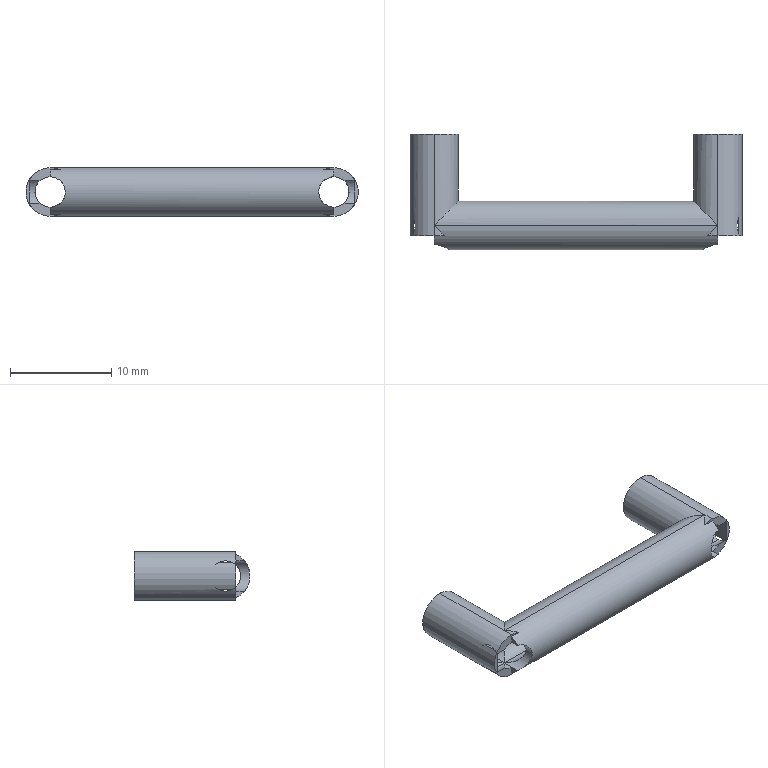Part | SolidWorks | features BaseBody 1 | 1 solid | 38 faces | box 32.8 x 11.4 x 4.8 mm | volume 474.136 mm3 | cylinder 28 | plane 10 | commonest cylinder face diameters 3 x18 4.8 x10
STEP:
#1=CARTESIAN_POINT('',(-14.,-15.,-2.4));
#2=VERTEX_POINT('',#1);
#3=CARTESIAN_POINT('',(-14.,-15.,2.4));
#4=VERTEX_POINT('',#3);
#5=CARTESIAN_POINT('',(-14.,-15.,-2.4));
#6=CARTESIAN_POINT('',(-9.2,-10.2,-2.4));
#7=CARTESIAN_POINT('',(-9.2,-10.2,2.4));
#8=CARTESIAN_POINT('',(-14.,-15.,2.4));
#9=(BOUNDED_CURVE()B_SPLINE_CURVE(3,(#5,#6,#7,#8),.UNSPECIFIED.,.F.,.F.)B_SPLINE_CURVE_WITH_KNOTS((4,4),(4.712,7.854),.UNSPECIFIED.)CURVE()GEOMETRIC_REPRESENTATION_ITEM()RATIONAL_B_SPLINE_CURVE((1.,0.3333,0.3333,1.))REPRESENTATION_ITEM(''));
#10=EDGE_CURVE('',#2,#4,#9,.T.);
#11=ORIENTED_EDGE('',*,*,#10,.T.);
#12=CARTESIAN_POINT('',(14.,-15.,2.4));
#13=VERTEX_POINT('',#12);
#14=CARTESIAN_POINT('',(-14.,-15.,2.4));
#15=DIRECTION('',(1.,0.,0.));
#16=VECTOR('',#15,1000.);
#17=LINE('',#14,#16);
#18=EDGE_CURVE('',#4,#13,#17,.T.);
#19=ORIENTED_EDGE('',*,*,#18,.T.);
#20=CARTESIAN_POINT('',(14.,-15.,-2.4));
#21=VERTEX_POINT('',#20);
#22=CARTESIAN_POINT('',(14.,-15.,2.4));
#23=CARTESIAN_POINT('',(9.2,-10.2,2.4));
#24=CARTESIAN_POINT('',(9.2,-10.2,-2.4));
#25=CARTESIAN_POINT('',(14.,-15.,-2.4));
#26=(BOUNDED_CURVE()B_SPLINE_CURVE(3,(#22,#23,#24,#25),.UNSPECIFIED.,.F.,.F.)B_SPLINE_CURVE_WITH_KNOTS((4,4),(4.712,7.854),.UNSPECIFIED.)CURVE()GEOMETRIC_REPRESENTATION_ITEM()RATIONAL_B_SPLINE_CURVE((1.,0.3333,0.3333,1.))REPRESENTATION_ITEM(''));
#27=EDGE_CURVE('',#13,#21,#26,.T.);
#28=ORIENTED_EDGE('',*,*,#27,.T.);
#29=CARTESIAN_POINT('',(-14.,-15.,-2.4));
#30=DIRECTION('',(1.,0.,0.));
#31=VECTOR('',#30,1000.);
#32=LINE('',#29,#31);
#33=EDGE_CURVE('',#2,#21,#32,.T.);
#34=ORIENTED_EDGE('',*,*,#33,.F.);
#35=EDGE_LOOP('',(#11,#19,#28,#34));
#36=FACE_OUTER_BOUND('',#35,.T.);
#37=CARTESIAN_POINT('',(-14.,-15.,0.));
#38=DIRECTION('',(1.,0.,0.));
#39=DIRECTION('',(0.,0.,-1.));
#40=AXIS2_PLACEMENT_3D('',#37,#38,#39);
#41=CYLINDRICAL_SURFACE('',#40,2.4);
#42=ADVANCED_FACE('',(#36),#41,.T.);
#43=CARTESIAN_POINT('',(-15.,-16.,-1.118));
#44=VERTEX_POINT('',#43);
#45=CARTESIAN_POINT('',(-14.,-16.,-1.5));
#46=VERTEX_POINT('',#45);
#47=CARTESIAN_POINT('',(-14.,-16.,0.));
#48=DIRECTION('',(0.,-1.,0.));
#49=DIRECTION('',(0.,0.,1.));
#50=AXIS2_PLACEMENT_3D('',#47,#48,#49);
#51=CIRCLE('',#50,1.5);
#52=EDGE_CURVE('',#44,#46,#51,.T.);
#53=ORIENTED_EDGE('',*,*,#52,.T.);
#54=CARTESIAN_POINT('',(-14.,-15.,-1.5));
#55=VERTEX_POINT('',#54);
#56=CARTESIAN_POINT('',(-14.,-18.,-1.5));
#57=DIRECTION('',(0.,1.,0.));
#58=VECTOR('',#57,1000.);
#59=LINE('',#56,#58);
#60=EDGE_CURVE('',#46,#55,#59,.T.);
#61=ORIENTED_EDGE('',*,*,#60,.T.);
#62=CARTESIAN_POINT('',(-14.,-15.,-1.5));
#63=CARTESIAN_POINT('',(-14.373,-15.373,-1.5));
#64=CARTESIAN_POINT('',(-14.722,-15.722,-1.367));
#65=CARTESIAN_POINT('',(-15.,-16.,-1.118));
#66=(BOUNDED_CURVE()B_SPLINE_CURVE(3,(#62,#63,#64,#65),.UNSPECIFIED.,.F.,.F.)B_SPLINE_CURVE_WITH_KNOTS((4,4),(1.571,2.301),.UNSPECIFIED.)CURVE()GEOMETRIC_REPRESENTATION_ITEM()RATIONAL_B_SPLINE_CURVE((1.,0.9561,0.9561,1.))REPRESENTATION_ITEM(''));
#67=EDGE_CURVE('',#55,#44,#66,.T.);
#68=ORIENTED_EDGE('',*,*,#67,.T.);
#69=EDGE_LOOP('',(#53,#61,#68));
#70=FACE_OUTER_BOUND('',#69,.T.);
#71=CARTESIAN_POINT('',(-14.,-18.,0.));
#72=DIRECTION('',(0.,1.,0.));
#73=DIRECTION('',(0.,0.,1.));
#74=AXIS2_PLACEMENT_3D('',#71,#72,#73);
#75=CYLINDRICAL_SURFACE('',#74,1.5);
#76=ADVANCED_FACE('',(#70),#75,.F.);
#77=ORIENTED_EDGE('',*,*,#60,.F.);
#78=CARTESIAN_POINT('',(-14.,-16.873,-1.5));
#79=VERTEX_POINT('',#78);
#80=CARTESIAN_POINT('',(-14.,-15.,-1.5));
#81=DIRECTION('',(0.,-1.,0.));
#82=VECTOR('',#81,1000.);
#83=LINE('',#80,#82);
#84=EDGE_CURVE('',#46,#79,#83,.T.);
#85=ORIENTED_EDGE('',*,*,#84,.T.);
#86=CARTESIAN_POINT('',(-14.,-16.873,1.5));
#87=VERTEX_POINT('',#86);
#88=CARTESIAN_POINT('',(-14.,-16.873,1.5));
#89=CARTESIAN_POINT('',(-13.898,-16.873,1.5));
#90=CARTESIAN_POINT('',(-13.798,-16.882,1.49));
#91=CARTESIAN_POINT('',(-13.603,-16.913,1.45));
#92=CARTESIAN_POINT('',(-13.507,-16.935,1.42));
#93=CARTESIAN_POINT('',(-13.238,-17.015,1.307));
#94=CARTESIAN_POINT('',(-13.077,-17.085,1.197));
#95=CARTESIAN_POINT('',(-12.874,-17.185,0.9958));
#96=CARTESIAN_POINT('',(-12.812,-17.218,0.921));
#97=CARTESIAN_POINT('',(-12.704,-17.278,0.7615));
#98=CARTESIAN_POINT('',(-12.658,-17.304,0.6768));
#99=CARTESIAN_POINT('',(-12.581,-17.35,0.4963));
#100=CARTESIAN_POINT('',(-12.551,-17.369,0.3994));
#101=CARTESIAN_POINT('',(-12.511,-17.393,0.2039));
#102=CARTESIAN_POINT('',(-12.5,-17.4,0.1043));
#103=CARTESIAN_POINT('',(-12.5,-17.4,-0.2004));
#104=CARTESIAN_POINT('',(-12.542,-17.373,-0.4024));
#105=CARTESIAN_POINT('',(-12.695,-17.282,-0.7658));
#106=CARTESIAN_POINT('',(-12.806,-17.218,-0.9283));
#107=CARTESIAN_POINT('',(-13.077,-17.085,-1.197));
#108=CARTESIAN_POINT('',(-13.237,-17.016,-1.306));
#109=CARTESIAN_POINT('',(-13.506,-16.936,-1.42));
#110=CARTESIAN_POINT('',(-13.602,-16.913,-1.45));
#111=CARTESIAN_POINT('',(-13.798,-16.882,-1.49));
#112=CARTESIAN_POINT('',(-13.898,-16.873,-1.5));
#113=CARTESIAN_POINT('',(-14.,-16.873,-1.5));
#114=B_SPLINE_CURVE_WITH_KNOTS('',3,(#88,#89,#90,#91,#92,#93,#94,#95,#96,#97,#98,#99,#100,#101,#102,#103,#104,#105,#106,#107,#108,#109,#110,#111,#112,#113),.UNSPECIFIED.,.F.,.F.,(4,2,2,2,2,2,2,2,2,2,2,2,4),(0.,0.0003015,0.0006029,0.001206,0.001507,0.001809,0.00211,0.002412,0.003015,0.003617,0.00422,0.004522,0.004823),.UNSPECIFIED.);
#115=EDGE_CURVE('',#87,#79,#114,.T.);
#116=ORIENTED_EDGE('',*,*,#115,.F.);
#117=CARTESIAN_POINT('',(-14.,-16.,1.5));
#118=VERTEX_POINT('',#117);
#119=CARTESIAN_POINT('',(-14.,-18.,1.5));
#120=DIRECTION('',(0.,-1.,0.));
#121=VECTOR('',#120,1000.);
#122=LINE('',#119,#121);
#123=EDGE_CURVE('',#118,#87,#122,.T.);
#124=ORIENTED_EDGE('',*,*,#123,.F.);
#125=CARTESIAN_POINT('',(-14.,-15.,1.5));
#126=VERTEX_POINT('',#125);
#127=CARTESIAN_POINT('',(-14.,-18.,1.5));
#128=DIRECTION('',(0.,1.,0.));
#129=VECTOR('',#128,1000.);
#130=LINE('',#127,#129);
#131=EDGE_CURVE('',#118,#126,#130,.T.);
#132=ORIENTED_EDGE('',*,*,#131,.T.);
#133=CARTESIAN_POINT('',(-14.,-15.,-1.5));
#134=CARTESIAN_POINT('',(-11.,-18.,-1.5));
#135=CARTESIAN_POINT('',(-11.,-18.,1.5));
#136=CARTESIAN_POINT('',(-14.,-15.,1.5));
#137=(BOUNDED_CURVE()B_SPLINE_CURVE(3,(#133,#134,#135,#136),.UNSPECIFIED.,.F.,.F.)B_SPLINE_CURVE_WITH_KNOTS((4,4),(4.712,7.854),.UNSPECIFIED.)CURVE()GEOMETRIC_REPRESENTATION_ITEM()RATIONAL_B_SPLINE_CURVE((1.,0.3333,0.3333,1.))REPRESENTATION_ITEM(''));
#138=EDGE_CURVE('',#55,#126,#137,.T.);
#139=ORIENTED_EDGE('',*,*,#138,.F.);
#140=EDGE_LOOP('',(#77,#85,#116,#124,#132,#139));
#141=FACE_OUTER_BOUND('',#140,.T.);
#142=CARTESIAN_POINT('',(-14.,-18.,0.));
#143=DIRECTION('',(0.,1.,0.));
#144=DIRECTION('',(0.,0.,1.));
#145=AXIS2_PLACEMENT_3D('',#142,#143,#144);
#146=CYLINDRICAL_SURFACE('',#145,1.5);
#147=ADVANCED_FACE('',(#141),#146,.F.);
#148=CARTESIAN_POINT('',(-13.,-16.,-2.182));
#149=VERTEX_POINT('',#148);
#150=CARTESIAN_POINT('',(-14.,-16.,-2.4));
#151=VERTEX_POINT('',#150);
#152=CARTESIAN_POINT('',(-14.,-16.,0.));
#153=DIRECTION('',(0.,1.,0.));
#154=DIRECTION('',(0.,0.,1.));
#155=AXIS2_PLACEMENT_3D('',#152,#153,#154);
#156=CIRCLE('',#155,2.4);
#157=EDGE_CURVE('',#149,#151,#156,.T.);
#158=ORIENTED_EDGE('',*,*,#157,.T.);
#159=CARTESIAN_POINT('',(-14.,-16.,-2.4));
#160=DIRECTION('',(0.,1.,0.));
#161=VECTOR('',#160,1000.);
#162=LINE('',#159,#161);
#163=EDGE_CURVE('',#151,#2,#162,.T.);
#164=ORIENTED_EDGE('',*,*,#163,.T.);
#165=CARTESIAN_POINT('',(-14.,-15.,-2.4));
#166=CARTESIAN_POINT('',(-13.654,-15.346,-2.4));
#167=CARTESIAN_POINT('',(-13.315,-15.685,-2.326));
#168=CARTESIAN_POINT('',(-13.,-16.,-2.182));
#169=(BOUNDED_CURVE()B_SPLINE_CURVE(3,(#165,#166,#167,#168),.UNSPECIFIED.,.F.,.F.)B_SPLINE_CURVE_WITH_KNOTS((4,4),(4.712,5.142),.UNSPECIFIED.)CURVE()GEOMETRIC_REPRESENTATION_ITEM()RATIONAL_B_SPLINE_CURVE((1.,0.9847,0.9847,1.))REPRESENTATION_ITEM(''));
#170=EDGE_CURVE('',#2,#149,#169,.T.);
#171=ORIENTED_EDGE('',*,*,#170,.T.);
#172=EDGE_LOOP('',(#158,#164,#171));
#173=FACE_OUTER_BOUND('',#172,.T.);
#174=CARTESIAN_POINT('',(-14.,-16.,0.));
#175=DIRECTION('',(0.,1.,0.));
#176=DIRECTION('',(0.,0.,1.));
#177=AXIS2_PLACEMENT_3D('',#174,#175,#176);
#178=CYLINDRICAL_SURFACE('',#177,2.4);
#179=ADVANCED_FACE('',(#173),#178,.T.);
#180=ORIENTED_EDGE('',*,*,#10,.F.);
#181=CARTESIAN_POINT('',(-14.,-6.,-2.4));
#182=VERTEX_POINT('',#181);
#183=CARTESIAN_POINT('',(-14.,-16.,-2.4));
#184=DIRECTION('',(0.,1.,0.));
#185=VECTOR('',#184,1000.);
#186=LINE('',#183,#185);
#187=EDGE_CURVE('',#2,#182,#186,.T.);
#188=ORIENTED_EDGE('',*,*,#187,.T.);
#189=CARTESIAN_POINT('',(-14.,-6.,2.4));
#190=VERTEX_POINT('',#189);
#191=CARTESIAN_POINT('',(-14.,-6.,0.));
#192=DIRECTION('',(0.,-1.,0.));
#193=DIRECTION('',(0.,0.,1.));
#194=AXIS2_PLACEMENT_3D('',#191,#192,#193);
#195=CIRCLE('',#194,2.4);
#196=EDGE_CURVE('',#182,#190,#195,.T.);
#197=ORIENTED_EDGE('',*,*,#196,.T.);
#198=CARTESIAN_POINT('',(-14.,-16.,2.4));
#199=DIRECTION('',(0.,1.,0.));
#200=VECTOR('',#199,1000.);
#201=LINE('',#198,#200);
#202=EDGE_CURVE('',#4,#190,#201,.T.);
#203=ORIENTED_EDGE('',*,*,#202,.F.);
#204=EDGE_LOOP('',(#180,#188,#197,#203));
#205=FACE_OUTER_BOUND('',#204,.T.);
#206=CARTESIAN_POINT('',(-14.,-16.,0.));
#207=DIRECTION('',(0.,1.,0.));
#208=DIRECTION('',(0.,0.,1.));
#209=AXIS2_PLACEMENT_3D('',#206,#207,#208);
#210=CYLINDRICAL_SURFACE('',#209,2.4);
#211=ADVANCED_FACE('',(#205),#210,.T.);
#212=ORIENTED_EDGE('',*,*,#163,.F.);
#213=CARTESIAN_POINT('',(-14.,-16.,2.4));
#214=VERTEX_POINT('',#213);
#215=CARTESIAN_POINT('',(-14.,-16.,0.));
#216=DIRECTION('',(0.,1.,0.));
#217=DIRECTION('',(0.,0.,1.));
#218=AXIS2_PLACEMENT_3D('',#215,#216,#217);
#219=CIRCLE('',#218,2.4);
#220=EDGE_CURVE('',#151,#214,#219,.T.);
#221=ORIENTED_EDGE('',*,*,#220,.T.);
#222=CARTESIAN_POINT('',(-14.,-16.,2.4));
#223=DIRECTION('',(0.,1.,0.));
#224=VECTOR('',#223,1000.);
#225=LINE('',#222,#224);
#226=EDGE_CURVE('',#214,#4,#225,.T.);
#227=ORIENTED_EDGE('',*,*,#226,.T.);
#228=ORIENTED_EDGE('',*,*,#202,.T.);
#229=CARTESIAN_POINT('',(-14.,-6.,0.));
#230=DIRECTION('',(0.,-1.,0.));
#231=DIRECTION('',(0.,0.,1.));
#232=AXIS2_PLACEMENT_3D('',#229,#230,#231);
#233=CIRCLE('',#232,2.4);
#234=EDGE_CURVE('',#190,#182,#233,.T.);
#235=ORIENTED_EDGE('',*,*,#234,.T.);
#236=ORIENTED_EDGE('',*,*,#187,.F.);
#237=EDGE_LOOP('',(#212,#221,#227,#228,#235,#236));
#238=FACE_OUTER_BOUND('',#237,.T.);
#239=CARTESIAN_POINT('',(-16.,-14.3,1.327));
#240=VERTEX_POINT('',#239);
#241=CARTESIAN_POINT('',(-16.,-15.7,1.327));
#242=VERTEX_POINT('',#241);
#243=CARTESIAN_POINT('',(-16.,-15.,1.327));
#244=DIRECTION('',(0.,-1.,0.));
#245=VECTOR('',#244,1000.);
#246=LINE('',#243,#245);
#247=EDGE_CURVE('',#240,#242,#246,.T.);
#248=ORIENTED_EDGE('',*,*,#247,.F.);
#249=CARTESIAN_POINT('',(-15.873,-15.,1.5));
#250=VERTEX_POINT('',#249);
#251=CARTESIAN_POINT('',(-16.,-14.3,1.327));
#252=CARTESIAN_POINT('',(-15.963,-14.405,1.382));
#253=CARTESIAN_POINT('',(-15.931,-14.517,1.425));
#254=CARTESIAN_POINT('',(-15.886,-14.753,1.485));
#255=CARTESIAN_POINT('',(-15.873,-14.877,1.5));
#256=CARTESIAN_POINT('',(-15.873,-15.,1.5));
#257=B_SPLINE_CURVE_WITH_KNOTS('',3,(#251,#252,#253,#254,#255,#256),.UNSPECIFIED.,.F.,.F.,(4,2,4),(0.,0.00037,0.0007401),.UNSPECIFIED.);
#258=EDGE_CURVE('',#240,#250,#257,.T.);
#259=ORIENTED_EDGE('',*,*,#258,.T.);
#260=CARTESIAN_POINT('',(-15.873,-15.,1.5));
#261=CARTESIAN_POINT('',(-15.873,-15.123,1.5));
#262=CARTESIAN_POINT('',(-15.886,-15.247,1.484));
#263=CARTESIAN_POINT('',(-15.931,-15.482,1.426));
#264=CARTESIAN_POINT('',(-15.963,-15.595,1.382));
#265=CARTESIAN_POINT('',(-16.,-15.7,1.327));
#266=B_SPLINE_CURVE_WITH_KNOTS('',3,(#260,#261,#262,#263,#264,#265),.UNSPECIFIED.,.F.,.F.,(4,2,4),(0.0007401,0.001109,0.001477),.UNSPECIFIED.);
#267=EDGE_CURVE('',#250,#242,#266,.T.);
#268=ORIENTED_EDGE('',*,*,#267,.T.);
#269=EDGE_LOOP('',(#248,#259,#268));
#270=FACE_BOUND('',#269,.T.);
#271=CARTESIAN_POINT('',(-16.,-15.7,-1.327));
#272=VERTEX_POINT('',#271);
#273=CARTESIAN_POINT('',(-15.873,-15.,-1.5));
#274=VERTEX_POINT('',#273);
#275=CARTESIAN_POINT('',(-16.,-15.7,-1.327));
#276=CARTESIAN_POINT('',(-15.963,-15.595,-1.382));
#277=CARTESIAN_POINT('',(-15.931,-15.483,-1.425));
#278=CARTESIAN_POINT('',(-15.886,-15.247,-1.485));
#279=CARTESIAN_POINT('',(-15.873,-15.123,-1.5));
#280=CARTESIAN_POINT('',(-15.873,-15.,-1.5));
#281=B_SPLINE_CURVE_WITH_KNOTS('',3,(#275,#276,#277,#278,#279,#280),.UNSPECIFIED.,.F.,.F.,(4,2,4),(0.,0.00037,0.0007401),.UNSPECIFIED.);
#282=EDGE_CURVE('',#272,#274,#281,.T.);
#283=ORIENTED_EDGE('',*,*,#282,.T.);
#284=CARTESIAN_POINT('',(-16.,-14.3,-1.327));
#285=VERTEX_POINT('',#284);
#286=CARTESIAN_POINT('',(-15.873,-15.,-1.5));
#287=CARTESIAN_POINT('',(-15.873,-14.877,-1.5));
#288=CARTESIAN_POINT('',(-15.886,-14.753,-1.484));
#289=CARTESIAN_POINT('',(-15.931,-14.518,-1.426));
#290=CARTESIAN_POINT('',(-15.963,-14.405,-1.382));
#291=CARTESIAN_POINT('',(-16.,-14.3,-1.327));
#292=B_SPLINE_CURVE_WITH_KNOTS('',3,(#286,#287,#288,#289,#290,#291),.UNSPECIFIED.,.F.,.F.,(4,2,4),(0.0007401,0.001109,0.001477),.UNSPECIFIED.);
#293=EDGE_CURVE('',#274,#285,#292,.T.);
#294=ORIENTED_EDGE('',*,*,#293,.T.);
#295=CARTESIAN_POINT('',(-16.,-16.,-1.327));
#296=DIRECTION('',(0.,-1.,0.));
#297=VECTOR('',#296,1000.);
#298=LINE('',#295,#297);
#299=EDGE_CURVE('',#285,#272,#298,.T.);
#300=ORIENTED_EDGE('',*,*,#299,.T.);
#301=EDGE_LOOP('',(#283,#294,#300));
#302=FACE_BOUND('',#301,.T.);
#303=CARTESIAN_POINT('',(-14.,-16.,0.));
#304=DIRECTION('',(0.,1.,0.));
#305=DIRECTION('',(0.,0.,1.));
#306=AXIS2_PLACEMENT_3D('',#303,#304,#305);
#307=CYLINDRICAL_SURFACE('',#306,2.4);
#308=ADVANCED_FACE('',(#238,#270,#302),#307,.T.);
#309=CARTESIAN_POINT('',(16.,-15.7,1.327));
#310=VERTEX_POINT('',#309);
#311=CARTESIAN_POINT('',(15.873,-15.,1.5));
#312=VERTEX_POINT('',#311);
#313=CARTESIAN_POINT('',(16.,-15.7,1.327));
#314=CARTESIAN_POINT('',(15.963,-15.595,1.382));
#315=CARTESIAN_POINT('',(15.931,-15.483,1.425));
#316=CARTESIAN_POINT('',(15.886,-15.247,1.485));
#317=CARTESIAN_POINT('',(15.873,-15.123,1.5));
#318=CARTESIAN_POINT('',(15.873,-15.,1.5));
#319=B_SPLINE_CURVE_WITH_KNOTS('',3,(#313,#314,#315,#316,#317,#318),.UNSPECIFIED.,.F.,.F.,(4,2,4),(0.,0.00037,0.0007401),.UNSPECIFIED.);
#320=EDGE_CURVE('',#310,#312,#319,.T.);
#321=ORIENTED_EDGE('',*,*,#320,.T.);
#322=CARTESIAN_POINT('',(16.,-14.3,1.327));
#323=VERTEX_POINT('',#322);
#324=CARTESIAN_POINT('',(15.873,-15.,1.5));
#325=CARTESIAN_POINT('',(15.873,-14.877,1.5));
#326=CARTESIAN_POINT('',(15.886,-14.753,1.484));
#327=CARTESIAN_POINT('',(15.931,-14.518,1.426));
#328=CARTESIAN_POINT('',(15.963,-14.405,1.382));
#329=CARTESIAN_POINT('',(16.,-14.3,1.327));
#330=B_SPLINE_CURVE_WITH_KNOTS('',3,(#324,#325,#326,#327,#328,#329),.UNSPECIFIED.,.F.,.F.,(4,2,4),(0.0007401,0.001109,0.001477),.UNSPECIFIED.);
#331=EDGE_CURVE('',#312,#323,#330,.T.);
#332=ORIENTED_EDGE('',*,*,#331,.T.);
#333=CARTESIAN_POINT('',(16.,-16.,1.327));
#334=DIRECTION('',(0.,-1.,0.));
#335=VECTOR('',#334,1000.);
#336=LINE('',#333,#335);
#337=EDGE_CURVE('',#323,#310,#336,.T.);
#338=ORIENTED_EDGE('',*,*,#337,.T.);
#339=EDGE_LOOP('',(#321,#332,#338));
#340=FACE_BOUND('',#339,.T.);
#341=CARTESIAN_POINT('',(16.,-14.3,-1.327));
#342=VERTEX_POINT('',#341);
#343=CARTESIAN_POINT('',(15.873,-15.,-1.5));
#344=VERTEX_POINT('',#343);
#345=CARTESIAN_POINT('',(16.,-14.3,-1.327));
#346=CARTESIAN_POINT('',(15.963,-14.405,-1.382));
#347=CARTESIAN_POINT('',(15.931,-14.517,-1.425));
#348=CARTESIAN_POINT('',(15.886,-14.753,-1.485));
#349=CARTESIAN_POINT('',(15.873,-14.877,-1.5));
#350=CARTESIAN_POINT('',(15.873,-15.,-1.5));
#351=B_SPLINE_CURVE_WITH_KNOTS('',3,(#345,#346,#347,#348,#349,#350),.UNSPECIFIED.,.F.,.F.,(4,2,4),(0.,0.00037,0.0007401),.UNSPECIFIED.);
#352=EDGE_CURVE('',#342,#344,#351,.T.);
#353=ORIENTED_EDGE('',*,*,#352,.T.);
#354=CARTESIAN_POINT('',(16.,-15.7,-1.327));
#355=VERTEX_POINT('',#354);
#356=CARTESIAN_POINT('',(15.873,-15.,-1.5));
#357=CARTESIAN_POINT('',(15.873,-15.123,-1.5));
#358=CARTESIAN_POINT('',(15.886,-15.247,-1.484));
#359=CARTESIAN_POINT('',(15.931,-15.482,-1.426));
#360=CARTESIAN_POINT('',(15.963,-15.595,-1.382));
#361=CARTESIAN_POINT('',(16.,-15.7,-1.327));
#362=B_SPLINE_CURVE_WITH_KNOTS('',3,(#356,#357,#358,#359,#360,#361),.UNSPECIFIED.,.F.,.F.,(4,2,4),(0.0007401,0.001109,0.001477),.UNSPECIFIED.);
#363=EDGE_CURVE('',#344,#355,#362,.T.);
#364=ORIENTED_EDGE('',*,*,#363,.T.);
#365=CARTESIAN_POINT('',(16.,-16.,-1.327));
#366=DIRECTION('',(0.,1.,0.));
#367=VECTOR('',#366,1000.);
#368=LINE('',#365,#367);
#369=EDGE_CURVE('',#355,#342,#368,.T.);
#370=ORIENTED_EDGE('',*,*,#369,.T.);
#371=EDGE_LOOP('',(#353,#364,#370));
#372=FACE_BOUND('',#371,.T.);
#373=CARTESIAN_POINT('',(14.,-16.,2.4));
#374=VERTEX_POINT('',#373);
#375=CARTESIAN_POINT('',(14.,-16.,-2.4));
#376=VERTEX_POINT('',#375);
#377=CARTESIAN_POINT('',(14.,-16.,0.));
#378=DIRECTION('',(0.,1.,0.));
#379=DIRECTION('',(0.,0.,1.));
#380=AXIS2_PLACEMENT_3D('',#377,#378,#379);
#381=CIRCLE('',#380,2.4);
#382=EDGE_CURVE('',#374,#376,#381,.T.);
#383=ORIENTED_EDGE('',*,*,#382,.T.);
#384=CARTESIAN_POINT('',(14.,-16.,-2.4));
#385=DIRECTION('',(0.,1.,0.));
#386=VECTOR('',#385,1000.);
#387=LINE('',#384,#386);
#388=EDGE_CURVE('',#376,#21,#387,.T.);
#389=ORIENTED_EDGE('',*,*,#388,.T.);
#390=CARTESIAN_POINT('',(14.,-6.,-2.4));
#391=VERTEX_POINT('',#390);
#392=CARTESIAN_POINT('',(14.,-16.,-2.4));
#393=DIRECTION('',(0.,1.,0.));
#394=VECTOR('',#393,1000.);
#395=LINE('',#392,#394);
#396=EDGE_CURVE('',#21,#391,#395,.T.);
#397=ORIENTED_EDGE('',*,*,#396,.T.);
#398=CARTESIAN_POINT('',(14.,-6.,2.4));
#399=VERTEX_POINT('',#398);
#400=CARTESIAN_POINT('',(14.,-6.,0.));
#401=DIRECTION('',(0.,-1.,0.));
#402=DIRECTION('',(0.,0.,1.));
#403=AXIS2_PLACEMENT_3D('',#400,#401,#402);
#404=CIRCLE('',#403,2.4);
#405=EDGE_CURVE('',#391,#399,#404,.T.);
#406=ORIENTED_EDGE('',*,*,#405,.T.);
#407=CARTESIAN_POINT('',(14.,-16.,2.4));
#408=DIRECTION('',(0.,1.,0.));
#409=VECTOR('',#408,1000.);
#410=LINE('',#407,#409);
#411=EDGE_CURVE('',#13,#399,#410,.T.);
#412=ORIENTED_EDGE('',*,*,#411,.F.);
#413=CARTESIAN_POINT('',(14.,-16.,2.4));
#414=DIRECTION('',(0.,1.,0.));
#415=VECTOR('',#414,1000.);
#416=LINE('',#413,#415);
#417=EDGE_CURVE('',#374,#13,#416,.T.);
#418=ORIENTED_EDGE('',*,*,#417,.F.);
#419=EDGE_LOOP('',(#383,#389,#397,#406,#412,#418));
#420=FACE_OUTER_BOUND('',#419,.T.);
#421=CARTESIAN_POINT('',(14.,-16.,0.));
#422=DIRECTION('',(0.,1.,0.));
#423=DIRECTION('',(0.,0.,1.));
#424=AXIS2_PLACEMENT_3D('',#421,#422,#423);
#425=CYLINDRICAL_SURFACE('',#424,2.4);
#426=ADVANCED_FACE('',(#340,#372,#420),#425,.T.);
#427=ORIENTED_EDGE('',*,*,#388,.F.);
#428=CARTESIAN_POINT('',(13.,-16.,-2.182));
#429=VERTEX_POINT('',#428);
#430=CARTESIAN_POINT('',(14.,-16.,0.));
#431=DIRECTION('',(0.,1.,0.));
#432=DIRECTION('',(0.,0.,1.));
#433=AXIS2_PLACEMENT_3D('',#430,#431,#432);
#434=CIRCLE('',#433,2.4);
#435=EDGE_CURVE('',#376,#429,#434,.T.);
#436=ORIENTED_EDGE('',*,*,#435,.T.);
#437=CARTESIAN_POINT('',(14.,-15.,-2.4));
#438=CARTESIAN_POINT('',(13.654,-15.346,-2.4));
#439=CARTESIAN_POINT('',(13.315,-15.685,-2.326));
#440=CARTESIAN_POINT('',(13.,-16.,-2.182));
#441=(BOUNDED_CURVE()B_SPLINE_CURVE(3,(#437,#438,#439,#440),.UNSPECIFIED.,.F.,.F.)B_SPLINE_CURVE_WITH_KNOTS((4,4),(1.571,2.001),.UNSPECIFIED.)CURVE()GEOMETRIC_REPRESENTATION_ITEM()RATIONAL_B_SPLINE_CURVE((1.,0.9847,0.9847,1.))REPRESENTATION_ITEM(''));
#442=EDGE_CURVE('',#21,#429,#441,.T.);
#443=ORIENTED_EDGE('',*,*,#442,.F.);
#444=EDGE_LOOP('',(#427,#436,#443));
#445=FACE_OUTER_BOUND('',#444,.T.);
#446=CARTESIAN_POINT('',(14.,-16.,0.));
#447=DIRECTION('',(0.,1.,0.));
#448=DIRECTION('',(0.,0.,1.));
#449=AXIS2_PLACEMENT_3D('',#446,#447,#448);
#450=CYLINDRICAL_SURFACE('',#449,2.4);
#451=ADVANCED_FACE('',(#445),#450,.T.);
#452=CARTESIAN_POINT('',(13.,-16.,2.182));
#453=VERTEX_POINT('',#452);
#454=CARTESIAN_POINT('',(14.,-16.,0.));
#455=DIRECTION('',(0.,1.,0.));
#456=DIRECTION('',(0.,0.,1.));
#457=AXIS2_PLACEMENT_3D('',#454,#455,#456);
#458=CIRCLE('',#457,2.4);
#459=EDGE_CURVE('',#453,#374,#458,.T.);
#460=ORIENTED_EDGE('',*,*,#459,.T.);
#461=ORIENTED_EDGE('',*,*,#417,.T.);
#462=CARTESIAN_POINT('',(13.,-16.,2.182));
#463=CARTESIAN_POINT('',(13.315,-15.685,2.326));
#464=CARTESIAN_POINT('',(13.654,-15.346,2.4));
#465=CARTESIAN_POINT('',(14.,-15.,2.4));
#466=(BOUNDED_CURVE()B_SPLINE_CURVE(3,(#462,#463,#464,#465),.UNSPECIFIED.,.F.,.F.)B_SPLINE_CURVE_WITH_KNOTS((4,4),(4.283,4.712),.UNSPECIFIED.)CURVE()GEOMETRIC_REPRESENTATION_ITEM()RATIONAL_B_SPLINE_CURVE((1.,0.9847,0.9847,1.))REPRESENTATION_ITEM(''));
#467=EDGE_CURVE('',#453,#13,#466,.T.);
#468=ORIENTED_EDGE('',*,*,#467,.F.);
#469=EDGE_LOOP('',(#460,#461,#468));
#470=FACE_OUTER_BOUND('',#469,.T.);
#471=CARTESIAN_POINT('',(14.,-16.,0.));
#472=DIRECTION('',(0.,1.,0.));
#473=DIRECTION('',(0.,0.,1.));
#474=AXIS2_PLACEMENT_3D('',#471,#472,#473);
#475=CYLINDRICAL_SURFACE('',#474,2.4);
#476=ADVANCED_FACE('',(#470),#475,.T.);
#477=CARTESIAN_POINT('',(14.,-16.,-1.5));
#478=VERTEX_POINT('',#477);
#479=CARTESIAN_POINT('',(14.,-16.873,-1.5));
#480=VERTEX_POINT('',#479);
#481=CARTESIAN_POINT('',(14.,-18.,-1.5));
#482=DIRECTION('',(0.,-1.,0.));
#483=VECTOR('',#482,1000.);
#484=LINE('',#481,#483);
#485=EDGE_CURVE('',#478,#480,#484,.T.);
#486=ORIENTED_EDGE('',*,*,#485,.F.);
#487=CARTESIAN_POINT('',(14.,-15.,-1.5));
#488=VERTEX_POINT('',#487);
#489=CARTESIAN_POINT('',(14.,-18.,-1.5));
#490=DIRECTION('',(0.,1.,0.));
#491=VECTOR('',#490,1000.);
#492=LINE('',#489,#491);
#493=EDGE_CURVE('',#478,#488,#492,.T.);
#494=ORIENTED_EDGE('',*,*,#493,.T.);
#495=CARTESIAN_POINT('',(14.,-15.,1.5));
#496=VERTEX_POINT('',#495);
#497=CARTESIAN_POINT('',(14.,-15.,1.5));
#498=CARTESIAN_POINT('',(11.,-18.,1.5));
#499=CARTESIAN_POINT('',(11.,-18.,-1.5));
#500=CARTESIAN_POINT('',(14.,-15.,-1.5));
#501=(BOUNDED_CURVE()B_SPLINE_CURVE(3,(#497,#498,#499,#500),.UNSPECIFIED.,.F.,.F.)B_SPLINE_CURVE_WITH_KNOTS((4,4),(1.571,4.712),.UNSPECIFIED.)CURVE()GEOMETRIC_REPRESENTATION_ITEM()RATIONAL_B_SPLINE_CURVE((1.,0.3333,0.3333,1.))REPRESENTATION_ITEM(''));
#502=EDGE_CURVE('',#496,#488,#501,.T.);
#503=ORIENTED_EDGE('',*,*,#502,.F.);
#504=CARTESIAN_POINT('',(14.,-16.,1.5));
#505=VERTEX_POINT('',#504);
#506=CARTESIAN_POINT('',(14.,-18.,1.5));
#507=DIRECTION('',(0.,1.,0.));
#508=VECTOR('',#507,1000.);
#509=LINE('',#506,#508);
#510=EDGE_CURVE('',#505,#496,#509,.T.);
#511=ORIENTED_EDGE('',*,*,#510,.F.);
#512=CARTESIAN_POINT('',(14.,-16.873,1.5));
#513=VERTEX_POINT('',#512);
#514=CARTESIAN_POINT('',(14.,-15.,1.5));
#515=DIRECTION('',(0.,1.,0.));
#516=VECTOR('',#515,1000.);
#517=LINE('',#514,#516);
#518=EDGE_CURVE('',#513,#505,#517,.T.);
#519=ORIENTED_EDGE('',*,*,#518,.F.);
#520=CARTESIAN_POINT('',(14.,-16.873,-1.5));
#521=CARTESIAN_POINT('',(13.898,-16.873,-1.5));
#522=CARTESIAN_POINT('',(13.798,-16.882,-1.49));
#523=CARTESIAN_POINT('',(13.603,-16.913,-1.45));
#524=CARTESIAN_POINT('',(13.507,-16.935,-1.42));
#525=CARTESIAN_POINT('',(13.238,-17.015,-1.307));
#526=CARTESIAN_POINT('',(13.077,-17.085,-1.197));
#527=CARTESIAN_POINT('',(12.874,-17.185,-0.9958));
#528=CARTESIAN_POINT('',(12.812,-17.218,-0.921));
#529=CARTESIAN_POINT('',(12.704,-17.278,-0.7615));
#530=CARTESIAN_POINT('',(12.658,-17.304,-0.6768));
#531=CARTESIAN_POINT('',(12.581,-17.35,-0.4963));
#532=CARTESIAN_POINT('',(12.551,-17.369,-0.3994));
#533=CARTESIAN_POINT('',(12.511,-17.393,-0.2039));
#534=CARTESIAN_POINT('',(12.5,-17.4,-0.1043));
#535=CARTESIAN_POINT('',(12.5,-17.4,0.2004));
#536=CARTESIAN_POINT('',(12.542,-17.373,0.4024));
#537=CARTESIAN_POINT('',(12.695,-17.282,0.7658));
#538=CARTESIAN_POINT('',(12.806,-17.218,0.9283));
#539=CARTESIAN_POINT('',(13.077,-17.085,1.197));
#540=CARTESIAN_POINT('',(13.237,-17.016,1.306));
#541=CARTESIAN_POINT('',(13.506,-16.936,1.42));
#542=CARTESIAN_POINT('',(13.602,-16.913,1.45));
#543=CARTESIAN_POINT('',(13.798,-16.882,1.49));
#544=CARTESIAN_POINT('',(13.898,-16.873,1.5));
#545=CARTESIAN_POINT('',(14.,-16.873,1.5));
#546=B_SPLINE_CURVE_WITH_KNOTS('',3,(#520,#521,#522,#523,#524,#525,#526,#527,#528,#529,#530,#531,#532,#533,#534,#535,#536,#537,#538,#539,#540,#541,#542,#543,#544,#545),.UNSPECIFIED.,.F.,.F.,(4,2,2,2,2,2,2,2,2,2,2,2,4),(0.,0.0003015,0.0006029,0.001206,0.001507,0.001809,0.00211,0.002412,0.003015,0.003617,0.00422,0.004522,0.004823),.UNSPECIFIED.);
#547=EDGE_CURVE('',#480,#513,#546,.T.);
#548=ORIENTED_EDGE('',*,*,#547,.F.);
#549=EDGE_LOOP('',(#486,#494,#503,#511,#519,#548));
#550=FACE_OUTER_BOUND('',#549,.T.);
#551=CARTESIAN_POINT('',(14.,-18.,0.));
#552=DIRECTION('',(0.,1.,0.));
#553=DIRECTION('',(0.,0.,1.));
#554=AXIS2_PLACEMENT_3D('',#551,#552,#553);
#555=CYLINDRICAL_SURFACE('',#554,1.5);
#556=ADVANCED_FACE('',(#550),#555,.F.);
#557=CARTESIAN_POINT('',(15.,-16.,1.118));
#558=VERTEX_POINT('',#557);
#559=CARTESIAN_POINT('',(14.,-16.,0.));
#560=DIRECTION('',(0.,1.,0.));
#561=DIRECTION('',(0.,0.,1.));
#562=AXIS2_PLACEMENT_3D('',#559,#560,#561);
#563=CIRCLE('',#562,1.5);
#564=EDGE_CURVE('',#505,#558,#563,.T.);
#565=ORIENTED_EDGE('',*,*,#564,.F.);
#566=ORIENTED_EDGE('',*,*,#510,.T.);
#567=CARTESIAN_POINT('',(14.,-15.,1.5));
#568=CARTESIAN_POINT('',(14.373,-15.373,1.5));
#569=CARTESIAN_POINT('',(14.722,-15.722,1.367));
#570=CARTESIAN_POINT('',(15.,-16.,1.118));
#571=(BOUNDED_CURVE()B_SPLINE_CURVE(3,(#567,#568,#569,#570),.UNSPECIFIED.,.F.,.F.)B_SPLINE_CURVE_WITH_KNOTS((4,4),(1.571,2.301),.UNSPECIFIED.)CURVE()GEOMETRIC_REPRESENTATION_ITEM()RATIONAL_B_SPLINE_CURVE((1.,0.9561,0.9561,1.))REPRESENTATION_ITEM(''));
#572=EDGE_CURVE('',#496,#558,#571,.T.);
#573=ORIENTED_EDGE('',*,*,#572,.T.);
#574=EDGE_LOOP('',(#565,#566,#573));
#575=FACE_OUTER_BOUND('',#574,.T.);
#576=CARTESIAN_POINT('',(14.,-18.,0.));
#577=DIRECTION('',(0.,1.,0.));
#578=DIRECTION('',(0.,0.,1.));
#579=AXIS2_PLACEMENT_3D('',#576,#577,#578);
#580=CYLINDRICAL_SURFACE('',#579,1.5);
#581=ADVANCED_FACE('',(#575),#580,.F.);
#582=ORIENTED_EDGE('',*,*,#138,.T.);
#583=CARTESIAN_POINT('',(-16.,-15.,1.5));
#584=DIRECTION('',(1.,0.,0.));
#585=VECTOR('',#584,1000.);
#586=LINE('',#583,#585);
#587=EDGE_CURVE('',#126,#496,#586,.T.);
#588=ORIENTED_EDGE('',*,*,#587,.T.);
#589=ORIENTED_EDGE('',*,*,#502,.T.);
#590=CARTESIAN_POINT('',(-16.,-15.,-1.5));
#591=DIRECTION('',(1.,0.,0.));
#592=VECTOR('',#591,1000.);
#593=LINE('',#590,#592);
#594=EDGE_CURVE('',#55,#488,#593,.T.);
#595=ORIENTED_EDGE('',*,*,#594,.F.);
#596=EDGE_LOOP('',(#582,#588,#589,#595));
#597=FACE_OUTER_BOUND('',#596,.T.);
#598=CARTESIAN_POINT('',(-16.,-15.,0.));
#599=DIRECTION('',(1.,0.,0.));
#600=DIRECTION('',(0.,0.,-1.));
#601=AXIS2_PLACEMENT_3D('',#598,#599,#600);
#602=CYLINDRICAL_SURFACE('',#601,1.5);
#603=ADVANCED_FACE('',(#597),#602,.F.);
#604=ORIENTED_EDGE('',*,*,#267,.F.);
#605=CARTESIAN_POINT('',(-16.,-15.,1.5));
#606=DIRECTION('',(1.,0.,0.));
#607=VECTOR('',#606,1000.);
#608=LINE('',#605,#607);
#609=EDGE_CURVE('',#250,#126,#608,.T.);
#610=ORIENTED_EDGE('',*,*,#609,.T.);
#611=CARTESIAN_POINT('',(-15.,-16.,1.118));
#612=VERTEX_POINT('',#611);
#613=CARTESIAN_POINT('',(-15.,-16.,1.118));
#614=CARTESIAN_POINT('',(-14.722,-15.722,1.367));
#615=CARTESIAN_POINT('',(-14.373,-15.373,1.5));
#616=CARTESIAN_POINT('',(-14.,-15.,1.5));
#617=(BOUNDED_CURVE()B_SPLINE_CURVE(3,(#613,#614,#615,#616),.UNSPECIFIED.,.F.,.F.)B_SPLINE_CURVE_WITH_KNOTS((4,4),(3.983,4.712),.UNSPECIFIED.)CURVE()GEOMETRIC_REPRESENTATION_ITEM()RATIONAL_B_SPLINE_CURVE((1.,0.9561,0.9561,1.))REPRESENTATION_ITEM(''));
#618=EDGE_CURVE('',#612,#126,#617,.T.);
#619=ORIENTED_EDGE('',*,*,#618,.F.);
#620=CARTESIAN_POINT('',(-16.,-16.,1.118));
#621=VERTEX_POINT('',#620);
#622=CARTESIAN_POINT('',(-16.,-16.,1.118));
#623=DIRECTION('',(1.,0.,0.));
#624=VECTOR('',#623,1000.);
#625=LINE('',#622,#624);
#626=EDGE_CURVE('',#621,#612,#625,.T.);
#627=ORIENTED_EDGE('',*,*,#626,.F.);
#628=CARTESIAN_POINT('',(-16.,-15.,0.));
#629=DIRECTION('',(1.,0.,0.));
#630=DIRECTION('',(0.,0.,-1.));
#631=AXIS2_PLACEMENT_3D('',#628,#629,#630);
#632=CIRCLE('',#631,1.5);
#633=EDGE_CURVE('',#242,#621,#632,.T.);
#634=ORIENTED_EDGE('',*,*,#633,.F.);
#635=EDGE_LOOP('',(#604,#610,#619,#627,#634));
#636=FACE_OUTER_BOUND('',#635,.T.);
#637=CARTESIAN_POINT('',(-16.,-15.,0.));
#638=DIRECTION('',(1.,0.,0.));
#639=DIRECTION('',(0.,0.,-1.));
#640=AXIS2_PLACEMENT_3D('',#637,#638,#639);
#641=CYLINDRICAL_SURFACE('',#640,1.5);
#642=ADVANCED_FACE('',(#636),#641,.F.);
#643=ORIENTED_EDGE('',*,*,#609,.F.);
#644=ORIENTED_EDGE('',*,*,#258,.F.);
#645=CARTESIAN_POINT('',(-16.,-15.,0.));
#646=DIRECTION('',(1.,0.,0.));
#647=DIRECTION('',(0.,0.,-1.));
#648=AXIS2_PLACEMENT_3D('',#645,#646,#647);
#649=CIRCLE('',#648,1.5);
#650=EDGE_CURVE('',#285,#240,#649,.T.);
#651=ORIENTED_EDGE('',*,*,#650,.F.);
#652=ORIENTED_EDGE('',*,*,#293,.F.);
#653=CARTESIAN_POINT('',(-16.,-15.,-1.5));
#654=DIRECTION('',(1.,0.,0.));
#655=VECTOR('',#654,1000.);
#656=LINE('',#653,#655);
#657=EDGE_CURVE('',#274,#55,#656,.T.);
#658=ORIENTED_EDGE('',*,*,#657,.T.);
#659=CARTESIAN_POINT('',(-14.,-15.,1.5));
#660=CARTESIAN_POINT('',(-17.,-12.,1.5));
#661=CARTESIAN_POINT('',(-17.,-12.,-1.5));
#662=CARTESIAN_POINT('',(-14.,-15.,-1.5));
#663=(BOUNDED_CURVE()B_SPLINE_CURVE(3,(#659,#660,#661,#662),.UNSPECIFIED.,.F.,.F.)B_SPLINE_CURVE_WITH_KNOTS((4,4),(4.712,7.854),.UNSPECIFIED.)CURVE()GEOMETRIC_REPRESENTATION_ITEM()RATIONAL_B_SPLINE_CURVE((1.,0.3333,0.3333,1.))REPRESENTATION_ITEM(''));
#664=EDGE_CURVE('',#126,#55,#663,.T.);
#665=ORIENTED_EDGE('',*,*,#664,.F.);
#666=EDGE_LOOP('',(#643,#644,#651,#652,#658,#665));
#667=FACE_OUTER_BOUND('',#666,.T.);
#668=CARTESIAN_POINT('',(-16.,-15.,0.));
#669=DIRECTION('',(1.,0.,0.));
#670=DIRECTION('',(0.,0.,-1.));
#671=AXIS2_PLACEMENT_3D('',#668,#669,#670);
#672=CYLINDRICAL_SURFACE('',#671,1.5);
#673=ADVANCED_FACE('',(#667),#672,.F.);
#674=ORIENTED_EDGE('',*,*,#664,.T.);
#675=CARTESIAN_POINT('',(-14.,-6.,-1.5));
#676=VERTEX_POINT('',#675);
#677=CARTESIAN_POINT('',(-14.,-18.,-1.5));
#678=DIRECTION('',(0.,1.,0.));
#679=VECTOR('',#678,1000.);
#680=LINE('',#677,#679);
#681=EDGE_CURVE('',#55,#676,#680,.T.);
#682=ORIENTED_EDGE('',*,*,#681,.T.);
#683=CARTESIAN_POINT('',(-14.,-6.,1.5));
#684=VERTEX_POINT('',#683);
#685=CARTESIAN_POINT('',(-14.,-6.,0.));
#686=DIRECTION('',(0.,-1.,0.));
#687=DIRECTION('',(0.,0.,1.));
#688=AXIS2_PLACEMENT_3D('',#685,#686,#687);
#689=CIRCLE('',#688,1.5);
#690=EDGE_CURVE('',#684,#676,#689,.T.);
#691=ORIENTED_EDGE('',*,*,#690,.F.);
#692=CARTESIAN_POINT('',(-14.,-18.,1.5));
#693=DIRECTION('',(0.,1.,0.));
#694=VECTOR('',#693,1000.);
#695=LINE('',#692,#694);
#696=EDGE_CURVE('',#126,#684,#695,.T.);
#697=ORIENTED_EDGE('',*,*,#696,.F.);
#698=EDGE_LOOP('',(#674,#682,#691,#697));
#699=FACE_OUTER_BOUND('',#698,.T.);
#700=CARTESIAN_POINT('',(-14.,-18.,0.));
#701=DIRECTION('',(0.,1.,0.));
#702=DIRECTION('',(0.,0.,1.));
#703=AXIS2_PLACEMENT_3D('',#700,#701,#702);
#704=CYLINDRICAL_SURFACE('',#703,1.5);
#705=ADVANCED_FACE('',(#699),#704,.F.);
#706=CARTESIAN_POINT('',(14.,-15.,1.5));
#707=CARTESIAN_POINT('',(11.,-12.,1.5));
#708=CARTESIAN_POINT('',(11.,-12.,-1.5));
#709=CARTESIAN_POINT('',(14.,-15.,-1.5));
#710=(BOUNDED_CURVE()B_SPLINE_CURVE(3,(#706,#707,#708,#709),.UNSPECIFIED.,.F.,.F.)B_SPLINE_CURVE_WITH_KNOTS((4,4),(4.712,7.854),.UNSPECIFIED.)CURVE()GEOMETRIC_REPRESENTATION_ITEM()RATIONAL_B_SPLINE_CURVE((1.,0.3333,0.3333,1.))REPRESENTATION_ITEM(''));
#711=EDGE_CURVE('',#496,#488,#710,.T.);
#712=ORIENTED_EDGE('',*,*,#711,.T.);
#713=CARTESIAN_POINT('',(14.,-6.,-1.5));
#714=VERTEX_POINT('',#713);
#715=CARTESIAN_POINT('',(14.,-18.,-1.5));
#716=DIRECTION('',(0.,1.,0.));
#717=VECTOR('',#716,1000.);
#718=LINE('',#715,#717);
#719=EDGE_CURVE('',#488,#714,#718,.T.);
#720=ORIENTED_EDGE('',*,*,#719,.T.);
#721=CARTESIAN_POINT('',(14.,-6.,1.5));
#722=VERTEX_POINT('',#721);
#723=CARTESIAN_POINT('',(14.,-6.,0.));
#724=DIRECTION('',(0.,-1.,0.));
#725=DIRECTION('',(0.,0.,1.));
#726=AXIS2_PLACEMENT_3D('',#723,#724,#725);
#727=CIRCLE('',#726,1.5);
#728=EDGE_CURVE('',#722,#714,#727,.T.);
#729=ORIENTED_EDGE('',*,*,#728,.F.);
#730=CARTESIAN_POINT('',(14.,-18.,1.5));
#731=DIRECTION('',(0.,1.,0.));
#732=VECTOR('',#731,1000.);
#733=LINE('',#730,#732);
#734=EDGE_CURVE('',#496,#722,#733,.T.);
#735=ORIENTED_EDGE('',*,*,#734,.F.);
#736=EDGE_LOOP('',(#712,#720,#729,#735));
#737=FACE_OUTER_BOUND('',#736,.T.);
#738=CARTESIAN_POINT('',(14.,-18.,0.));
#739=DIRECTION('',(0.,1.,0.));
#740=DIRECTION('',(0.,0.,1.));
#741=AXIS2_PLACEMENT_3D('',#738,#739,#740);
#742=CYLINDRICAL_SURFACE('',#741,1.5);
#743=ADVANCED_FACE('',(#737),#742,.F.);
#744=ORIENTED_EDGE('',*,*,#572,.F.);
#745=CARTESIAN_POINT('',(-16.,-15.,1.5));
#746=DIRECTION('',(1.,0.,0.));
#747=VECTOR('',#746,1000.);
#748=LINE('',#745,#747);
#749=EDGE_CURVE('',#496,#312,#748,.T.);
#750=ORIENTED_EDGE('',*,*,#749,.T.);
#751=ORIENTED_EDGE('',*,*,#320,.F.);
#752=CARTESIAN_POINT('',(16.,-16.,1.118));
#753=VERTEX_POINT('',#752);
#754=CARTESIAN_POINT('',(16.,-15.,0.));
#755=DIRECTION('',(-1.,0.,0.));
#756=DIRECTION('',(0.,0.,-1.));
#757=AXIS2_PLACEMENT_3D('',#754,#755,#756);
#758=CIRCLE('',#757,1.5);
#759=EDGE_CURVE('',#753,#310,#758,.T.);
#760=ORIENTED_EDGE('',*,*,#759,.F.);
#761=CARTESIAN_POINT('',(14.,-16.,1.118));
#762=DIRECTION('',(-1.,0.,0.));
#763=VECTOR('',#762,1000.);
#764=LINE('',#761,#763);
#765=EDGE_CURVE('',#753,#558,#764,.T.);
#766=ORIENTED_EDGE('',*,*,#765,.T.);
#767=EDGE_LOOP('',(#744,#750,#751,#760,#766));
#768=FACE_OUTER_BOUND('',#767,.T.);
#769=CARTESIAN_POINT('',(-16.,-15.,0.));
#770=DIRECTION('',(1.,0.,0.));
#771=DIRECTION('',(0.,0.,-1.));
#772=AXIS2_PLACEMENT_3D('',#769,#770,#771);
#773=CYLINDRICAL_SURFACE('',#772,1.5);
#774=ADVANCED_FACE('',(#768),#773,.F.);
#775=ORIENTED_EDGE('',*,*,#749,.F.);
#776=CARTESIAN_POINT('',(14.,-15.,1.5));
#777=CARTESIAN_POINT('',(17.,-12.,1.5));
#778=CARTESIAN_POINT('',(17.,-12.,-1.5));
#779=CARTESIAN_POINT('',(14.,-15.,-1.5));
#780=(BOUNDED_CURVE()B_SPLINE_CURVE(3,(#776,#777,#778,#779),.UNSPECIFIED.,.F.,.F.)B_SPLINE_CURVE_WITH_KNOTS((4,4),(4.712,7.854),.UNSPECIFIED.)CURVE()GEOMETRIC_REPRESENTATION_ITEM()RATIONAL_B_SPLINE_CURVE((1.,0.3333,0.3333,1.))REPRESENTATION_ITEM(''));
#781=EDGE_CURVE('',#496,#488,#780,.T.);
#782=ORIENTED_EDGE('',*,*,#781,.T.);
#783=CARTESIAN_POINT('',(-16.,-15.,-1.5));
#784=DIRECTION('',(1.,0.,0.));
#785=VECTOR('',#784,1000.);
#786=LINE('',#783,#785);
#787=EDGE_CURVE('',#488,#344,#786,.T.);
#788=ORIENTED_EDGE('',*,*,#787,.T.);
#789=ORIENTED_EDGE('',*,*,#352,.F.);
#790=CARTESIAN_POINT('',(16.,-15.,0.));
#791=DIRECTION('',(1.,0.,0.));
#792=DIRECTION('',(0.,0.,-1.));
#793=AXIS2_PLACEMENT_3D('',#790,#791,#792);
#794=CIRCLE('',#793,1.5);
#795=EDGE_CURVE('',#342,#323,#794,.T.);
#796=ORIENTED_EDGE('',*,*,#795,.T.);
#797=ORIENTED_EDGE('',*,*,#331,.F.);
#798=EDGE_LOOP('',(#775,#782,#788,#789,#796,#797));
#799=FACE_OUTER_BOUND('',#798,.T.);
#800=CARTESIAN_POINT('',(-16.,-15.,0.));
#801=DIRECTION('',(1.,0.,0.));
#802=DIRECTION('',(0.,0.,-1.));
#803=AXIS2_PLACEMENT_3D('',#800,#801,#802);
#804=CYLINDRICAL_SURFACE('',#803,1.5);
#805=ADVANCED_FACE('',(#799),#804,.F.);
#806=ORIENTED_EDGE('',*,*,#18,.F.);
#807=CARTESIAN_POINT('',(-13.,-16.,2.182));
#808=VERTEX_POINT('',#807);
#809=CARTESIAN_POINT('',(-13.,-16.,2.182));
#810=CARTESIAN_POINT('',(-13.315,-15.685,2.326));
#811=CARTESIAN_POINT('',(-13.654,-15.346,2.4));
#812=CARTESIAN_POINT('',(-14.,-15.,2.4));
#813=(BOUNDED_CURVE()B_SPLINE_CURVE(3,(#809,#810,#811,#812),.UNSPECIFIED.,.F.,.F.)B_SPLINE_CURVE_WITH_KNOTS((4,4),(1.141,1.571),.UNSPECIFIED.)CURVE()GEOMETRIC_REPRESENTATION_ITEM()RATIONAL_B_SPLINE_CURVE((1.,0.9847,0.9847,1.))REPRESENTATION_ITEM(''));
#814=EDGE_CURVE('',#808,#4,#813,.T.);
#815=ORIENTED_EDGE('',*,*,#814,.F.);
#816=CARTESIAN_POINT('',(-14.,-16.,2.182));
#817=VERTEX_POINT('',#816);
#818=CARTESIAN_POINT('',(-14.,-16.,2.182));
#819=DIRECTION('',(-1.,0.,0.));
#820=VECTOR('',#819,1000.);
#821=LINE('',#818,#820);
#822=EDGE_CURVE('',#808,#817,#821,.T.);
#823=ORIENTED_EDGE('',*,*,#822,.T.);
#824=CARTESIAN_POINT('',(-14.,-15.,0.));
#825=DIRECTION('',(1.,0.,0.));
#826=DIRECTION('',(0.,0.,-1.));
#827=AXIS2_PLACEMENT_3D('',#824,#825,#826);
#828=CIRCLE('',#827,2.4);
#829=EDGE_CURVE('',#817,#87,#828,.T.);
#830=ORIENTED_EDGE('',*,*,#829,.T.);
#831=ORIENTED_EDGE('',*,*,#115,.T.);
#832=CARTESIAN_POINT('',(-14.,-16.,-2.182));
#833=VERTEX_POINT('',#832);
#834=CARTESIAN_POINT('',(-14.,-15.,0.));
#835=DIRECTION('',(1.,0.,0.));
#836=DIRECTION('',(0.,0.,-1.));
#837=AXIS2_PLACEMENT_3D('',#834,#835,#836);
#838=CIRCLE('',#837,2.4);
#839=EDGE_CURVE('',#79,#833,#838,.T.);
#840=ORIENTED_EDGE('',*,*,#839,.T.);
#841=CARTESIAN_POINT('',(-14.,-16.,-2.182));
#842=DIRECTION('',(1.,0.,0.));
#843=VECTOR('',#842,1000.);
#844=LINE('',#841,#843);
#845=EDGE_CURVE('',#833,#149,#844,.T.);
#846=ORIENTED_EDGE('',*,*,#845,.T.);
#847=ORIENTED_EDGE('',*,*,#170,.F.);
#848=ORIENTED_EDGE('',*,*,#33,.T.);
#849=ORIENTED_EDGE('',*,*,#442,.T.);
#850=CARTESIAN_POINT('',(14.,-16.,-2.182));
#851=VERTEX_POINT('',#850);
#852=CARTESIAN_POINT('',(14.,-16.,-2.182));
#853=DIRECTION('',(1.,0.,0.));
#854=VECTOR('',#853,1000.);
#855=LINE('',#852,#854);
#856=EDGE_CURVE('',#429,#851,#855,.T.);
#857=ORIENTED_EDGE('',*,*,#856,.T.);
#858=CARTESIAN_POINT('',(14.,-15.,0.));
#859=DIRECTION('',(-1.,0.,0.));
#860=DIRECTION('',(0.,0.,-1.));
#861=AXIS2_PLACEMENT_3D('',#858,#859,#860);
#862=CIRCLE('',#861,2.4);
#863=EDGE_CURVE('',#851,#480,#862,.T.);
#864=ORIENTED_EDGE('',*,*,#863,.T.);
#865=ORIENTED_EDGE('',*,*,#547,.T.);
#866=CARTESIAN_POINT('',(14.,-16.,2.182));
#867=VERTEX_POINT('',#866);
#868=CARTESIAN_POINT('',(14.,-15.,0.));
#869=DIRECTION('',(-1.,0.,0.));
#870=DIRECTION('',(0.,0.,-1.));
#871=AXIS2_PLACEMENT_3D('',#868,#869,#870);
#872=CIRCLE('',#871,2.4);
#873=EDGE_CURVE('',#513,#867,#872,.T.);
#874=ORIENTED_EDGE('',*,*,#873,.T.);
#875=CARTESIAN_POINT('',(14.,-16.,2.182));
#876=DIRECTION('',(-1.,0.,0.));
#877=VECTOR('',#876,1000.);
#878=LINE('',#875,#877);
#879=EDGE_CURVE('',#867,#453,#878,.T.);
#880=ORIENTED_EDGE('',*,*,#879,.T.);
#881=ORIENTED_EDGE('',*,*,#467,.T.);
#882=EDGE_LOOP('',(#806,#815,#823,#830,#831,#840,#846,#847,#848,#849,#857,#864,#865,#874,#880,#881));
#883=FACE_OUTER_BOUND('',#882,.T.);
#884=CARTESIAN_POINT('',(-14.,-15.,0.));
#885=DIRECTION('',(1.,0.,0.));
#886=DIRECTION('',(0.,0.,-1.));
#887=AXIS2_PLACEMENT_3D('',#884,#885,#886);
#888=CYLINDRICAL_SURFACE('',#887,2.4);
#889=ADVANCED_FACE('',(#883),#888,.T.);
#890=ORIENTED_EDGE('',*,*,#839,.F.);
#891=ORIENTED_EDGE('',*,*,#84,.F.);
#892=CARTESIAN_POINT('',(-14.,-16.,0.));
#893=DIRECTION('',(0.,0.,-1.));
#894=VECTOR('',#893,1000.);
#895=LINE('',#892,#894);
#896=EDGE_CURVE('',#46,#833,#895,.T.);
#897=ORIENTED_EDGE('',*,*,#896,.T.);
#898=EDGE_LOOP('',(#890,#891,#897));
#899=FACE_OUTER_BOUND('',#898,.T.);
#900=CARTESIAN_POINT('',(-14.,-15.,0.));
#901=DIRECTION('',(1.,0.,0.));
#902=DIRECTION('',(0.,0.,-1.));
#903=AXIS2_PLACEMENT_3D('',#900,#901,#902);
#904=PLANE('',#903);
#905=ADVANCED_FACE('',(#899),#904,.F.);
#906=ORIENTED_EDGE('',*,*,#131,.F.);
#907=CARTESIAN_POINT('',(-14.,-16.,0.));
#908=DIRECTION('',(0.,-1.,0.));
#909=DIRECTION('',(0.,0.,1.));
#910=AXIS2_PLACEMENT_3D('',#907,#908,#909);
#911=CIRCLE('',#910,1.5);
#912=EDGE_CURVE('',#118,#612,#911,.T.);
#913=ORIENTED_EDGE('',*,*,#912,.T.);
#914=ORIENTED_EDGE('',*,*,#618,.T.);
#915=EDGE_LOOP('',(#906,#913,#914));
#916=FACE_OUTER_BOUND('',#915,.T.);
#917=CARTESIAN_POINT('',(-14.,-18.,0.));
#918=DIRECTION('',(0.,1.,0.));
#919=DIRECTION('',(0.,0.,1.));
#920=AXIS2_PLACEMENT_3D('',#917,#918,#919);
#921=CYLINDRICAL_SURFACE('',#920,1.5);
#922=ADVANCED_FACE('',(#916),#921,.F.);
#923=ORIENTED_EDGE('',*,*,#829,.F.);
#924=CARTESIAN_POINT('',(-14.,-16.,0.));
#925=DIRECTION('',(0.,0.,-1.));
#926=VECTOR('',#925,1000.);
#927=LINE('',#924,#926);
#928=EDGE_CURVE('',#817,#118,#927,.T.);
#929=ORIENTED_EDGE('',*,*,#928,.T.);
#930=ORIENTED_EDGE('',*,*,#123,.T.);
#931=EDGE_LOOP('',(#923,#929,#930));
#932=FACE_OUTER_BOUND('',#931,.T.);
#933=CARTESIAN_POINT('',(-14.,-15.,0.));
#934=DIRECTION('',(1.,0.,0.));
#935=DIRECTION('',(0.,0.,-1.));
#936=AXIS2_PLACEMENT_3D('',#933,#934,#935);
#937=PLANE('',#936);
#938=ADVANCED_FACE('',(#932),#937,.F.);
#939=ORIENTED_EDGE('',*,*,#226,.F.);
#940=CARTESIAN_POINT('',(-14.,-16.,0.));
#941=DIRECTION('',(0.,1.,0.));
#942=DIRECTION('',(0.,0.,1.));
#943=AXIS2_PLACEMENT_3D('',#940,#941,#942);
#944=CIRCLE('',#943,2.4);
#945=EDGE_CURVE('',#214,#808,#944,.T.);
#946=ORIENTED_EDGE('',*,*,#945,.T.);
#947=ORIENTED_EDGE('',*,*,#814,.T.);
#948=EDGE_LOOP('',(#939,#946,#947));
#949=FACE_OUTER_BOUND('',#948,.T.);
#950=CARTESIAN_POINT('',(-14.,-16.,0.));
#951=DIRECTION('',(0.,1.,0.));
#952=DIRECTION('',(0.,0.,1.));
#953=AXIS2_PLACEMENT_3D('',#950,#951,#952);
#954=CYLINDRICAL_SURFACE('',#953,2.4);
#955=ADVANCED_FACE('',(#949),#954,.T.);
#956=ORIENTED_EDGE('',*,*,#396,.F.);
#957=ORIENTED_EDGE('',*,*,#27,.F.);
#958=ORIENTED_EDGE('',*,*,#411,.T.);
#959=CARTESIAN_POINT('',(14.,-6.,0.));
#960=DIRECTION('',(0.,-1.,0.));
#961=DIRECTION('',(0.,0.,1.));
#962=AXIS2_PLACEMENT_3D('',#959,#960,#961);
#963=CIRCLE('',#962,2.4);
#964=EDGE_CURVE('',#399,#391,#963,.T.);
#965=ORIENTED_EDGE('',*,*,#964,.T.);
#966=EDGE_LOOP('',(#956,#957,#958,#965));
#967=FACE_OUTER_BOUND('',#966,.T.);
#968=CARTESIAN_POINT('',(14.,-16.,0.));
#969=DIRECTION('',(0.,1.,0.));
#970=DIRECTION('',(0.,0.,1.));
#971=AXIS2_PLACEMENT_3D('',#968,#969,#970);
#972=CYLINDRICAL_SURFACE('',#971,2.4);
#973=ADVANCED_FACE('',(#967),#972,.T.);
#974=ORIENTED_EDGE('',*,*,#873,.F.);
#975=ORIENTED_EDGE('',*,*,#518,.T.);
#976=CARTESIAN_POINT('',(14.,-16.,0.));
#977=DIRECTION('',(0.,0.,1.));
#978=VECTOR('',#977,1000.);
#979=LINE('',#976,#978);
#980=EDGE_CURVE('',#505,#867,#979,.T.);
#981=ORIENTED_EDGE('',*,*,#980,.T.);
#982=EDGE_LOOP('',(#974,#975,#981));
#983=FACE_OUTER_BOUND('',#982,.T.);
#984=CARTESIAN_POINT('',(14.,-15.,0.));
#985=DIRECTION('',(1.,0.,0.));
#986=DIRECTION('',(0.,0.,-1.));
#987=AXIS2_PLACEMENT_3D('',#984,#985,#986);
#988=PLANE('',#987);
#989=ADVANCED_FACE('',(#983),#988,.T.);
#990=ORIENTED_EDGE('',*,*,#493,.F.);
#991=CARTESIAN_POINT('',(15.,-16.,-1.118));
#992=VERTEX_POINT('',#991);
#993=CARTESIAN_POINT('',(14.,-16.,0.));
#994=DIRECTION('',(0.,1.,0.));
#995=DIRECTION('',(0.,0.,1.));
#996=AXIS2_PLACEMENT_3D('',#993,#994,#995);
#997=CIRCLE('',#996,1.5);
#998=EDGE_CURVE('',#992,#478,#997,.T.);
#999=ORIENTED_EDGE('',*,*,#998,.F.);
#1000=CARTESIAN_POINT('',(15.,-16.,-1.118));
#1001=CARTESIAN_POINT('',(14.722,-15.722,-1.367));
#1002=CARTESIAN_POINT('',(14.373,-15.373,-1.5));
#1003=CARTESIAN_POINT('',(14.,-15.,-1.5));
#1004=(BOUNDED_CURVE()B_SPLINE_CURVE(3,(#1000,#1001,#1002,#1003),.UNSPECIFIED.,.F.,.F.)B_SPLINE_CURVE_WITH_KNOTS((4,4),(3.983,4.712),.UNSPECIFIED.)CURVE()GEOMETRIC_REPRESENTATION_ITEM()RATIONAL_B_SPLINE_CURVE((1.,0.9561,0.9561,1.))REPRESENTATION_ITEM(''));
#1005=EDGE_CURVE('',#992,#488,#1004,.T.);
#1006=ORIENTED_EDGE('',*,*,#1005,.T.);
#1007=EDGE_LOOP('',(#990,#999,#1006));
#1008=FACE_OUTER_BOUND('',#1007,.T.);
#1009=CARTESIAN_POINT('',(14.,-18.,0.));
#1010=DIRECTION('',(0.,1.,0.));
#1011=DIRECTION('',(0.,0.,1.));
#1012=AXIS2_PLACEMENT_3D('',#1009,#1010,#1011);
#1013=CYLINDRICAL_SURFACE('',#1012,1.5);
#1014=ADVANCED_FACE('',(#1008),#1013,.F.);
#1015=ORIENTED_EDGE('',*,*,#863,.F.);
#1016=CARTESIAN_POINT('',(14.,-16.,0.));
#1017=DIRECTION('',(0.,0.,1.));
#1018=VECTOR('',#1017,1000.);
#1019=LINE('',#1016,#1018);
#1020=EDGE_CURVE('',#851,#478,#1019,.T.);
#1021=ORIENTED_EDGE('',*,*,#1020,.T.);
#1022=ORIENTED_EDGE('',*,*,#485,.T.);
#1023=EDGE_LOOP('',(#1015,#1021,#1022));
#1024=FACE_OUTER_BOUND('',#1023,.T.);
#1025=CARTESIAN_POINT('',(14.,-15.,0.));
#1026=DIRECTION('',(1.,0.,0.));
#1027=DIRECTION('',(0.,0.,-1.));
#1028=AXIS2_PLACEMENT_3D('',#1025,#1026,#1027);
#1029=PLANE('',#1028);
#1030=ADVANCED_FACE('',(#1024),#1029,.T.);
#1031=ORIENTED_EDGE('',*,*,#587,.F.);
#1032=CARTESIAN_POINT('',(-14.,-15.,-1.5));
#1033=CARTESIAN_POINT('',(-11.,-12.,-1.5));
#1034=CARTESIAN_POINT('',(-11.,-12.,1.5));
#1035=CARTESIAN_POINT('',(-14.,-15.,1.5));
#1036=(BOUNDED_CURVE()B_SPLINE_CURVE(3,(#1032,#1033,#1034,#1035),.UNSPECIFIED.,.F.,.F.)B_SPLINE_CURVE_WITH_KNOTS((4,4),(4.712,7.854),.UNSPECIFIED.)CURVE()GEOMETRIC_REPRESENTATION_ITEM()RATIONAL_B_SPLINE_CURVE((1.,0.3333,0.3333,1.))REPRESENTATION_ITEM(''));
#1037=EDGE_CURVE('',#55,#126,#1036,.T.);
#1038=ORIENTED_EDGE('',*,*,#1037,.F.);
#1039=ORIENTED_EDGE('',*,*,#594,.T.);
#1040=ORIENTED_EDGE('',*,*,#711,.F.);
#1041=EDGE_LOOP('',(#1031,#1038,#1039,#1040));
#1042=FACE_OUTER_BOUND('',#1041,.T.);
#1043=CARTESIAN_POINT('',(-16.,-15.,0.));
#1044=DIRECTION('',(1.,0.,0.));
#1045=DIRECTION('',(0.,0.,-1.));
#1046=AXIS2_PLACEMENT_3D('',#1043,#1044,#1045);
#1047=CYLINDRICAL_SURFACE('',#1046,1.5);
#1048=ADVANCED_FACE('',(#1042),#1047,.F.);
#1049=ORIENTED_EDGE('',*,*,#657,.F.);
#1050=ORIENTED_EDGE('',*,*,#282,.F.);
#1051=CARTESIAN_POINT('',(-16.,-16.,-1.118));
#1052=VERTEX_POINT('',#1051);
#1053=CARTESIAN_POINT('',(-16.,-15.,0.));
#1054=DIRECTION('',(1.,0.,0.));
#1055=DIRECTION('',(0.,0.,-1.));
#1056=AXIS2_PLACEMENT_3D('',#1053,#1054,#1055);
#1057=CIRCLE('',#1056,1.5);
#1058=EDGE_CURVE('',#1052,#272,#1057,.T.);
#1059=ORIENTED_EDGE('',*,*,#1058,.F.);
#1060=CARTESIAN_POINT('',(-16.,-16.,-1.118));
#1061=DIRECTION('',(-1.,0.,0.));
#1062=VECTOR('',#1061,1000.);
#1063=LINE('',#1060,#1062);
#1064=EDGE_CURVE('',#44,#1052,#1063,.T.);
#1065=ORIENTED_EDGE('',*,*,#1064,.F.);
#1066=ORIENTED_EDGE('',*,*,#67,.F.);
#1067=EDGE_LOOP('',(#1049,#1050,#1059,#1065,#1066));
#1068=FACE_OUTER_BOUND('',#1067,.T.);
#1069=CARTESIAN_POINT('',(-16.,-15.,0.));
#1070=DIRECTION('',(1.,0.,0.));
#1071=DIRECTION('',(0.,0.,-1.));
#1072=AXIS2_PLACEMENT_3D('',#1069,#1070,#1071);
#1073=CYLINDRICAL_SURFACE('',#1072,1.5);
#1074=ADVANCED_FACE('',(#1068),#1073,.F.);
#1075=CARTESIAN_POINT('',(-16.,-16.,0.));
#1076=DIRECTION('',(0.,0.,-1.));
#1077=VECTOR('',#1076,1000.);
#1078=LINE('',#1075,#1077);
#1079=EDGE_CURVE('',#621,#1052,#1078,.T.);
#1080=ORIENTED_EDGE('',*,*,#1079,.T.);
#1081=ORIENTED_EDGE('',*,*,#1058,.T.);
#1082=ORIENTED_EDGE('',*,*,#299,.F.);
#1083=ORIENTED_EDGE('',*,*,#650,.T.);
#1084=ORIENTED_EDGE('',*,*,#247,.T.);
#1085=ORIENTED_EDGE('',*,*,#633,.T.);
#1086=EDGE_LOOP('',(#1080,#1081,#1082,#1083,#1084,#1085));
#1087=FACE_OUTER_BOUND('',#1086,.T.);
#1088=CARTESIAN_POINT('',(-16.,-15.,0.));
#1089=DIRECTION('',(1.,0.,0.));
#1090=DIRECTION('',(0.,0.,-1.));
#1091=AXIS2_PLACEMENT_3D('',#1088,#1089,#1090);
#1092=PLANE('',#1091);
#1093=ADVANCED_FACE('',(#1087),#1092,.T.);
#1094=ORIENTED_EDGE('',*,*,#1064,.T.);
#1095=ORIENTED_EDGE('',*,*,#1079,.F.);
#1096=ORIENTED_EDGE('',*,*,#626,.T.);
#1097=ORIENTED_EDGE('',*,*,#912,.F.);
#1098=ORIENTED_EDGE('',*,*,#928,.F.);
#1099=ORIENTED_EDGE('',*,*,#822,.F.);
#1100=ORIENTED_EDGE('',*,*,#945,.F.);
#1101=ORIENTED_EDGE('',*,*,#220,.F.);
#1102=ORIENTED_EDGE('',*,*,#157,.F.);
#1103=ORIENTED_EDGE('',*,*,#845,.F.);
#1104=ORIENTED_EDGE('',*,*,#896,.F.);
#1105=ORIENTED_EDGE('',*,*,#52,.F.);
#1106=EDGE_LOOP('',(#1094,#1095,#1096,#1097,#1098,#1099,#1100,#1101,#1102,#1103,#1104,#1105));
#1107=FACE_OUTER_BOUND('',#1106,.T.);
#1108=CARTESIAN_POINT('',(-14.,-16.,0.));
#1109=DIRECTION('',(0.,1.,0.));
#1110=DIRECTION('',(0.,0.,1.));
#1111=AXIS2_PLACEMENT_3D('',#1108,#1109,#1110);
#1112=PLANE('',#1111);
#1113=ADVANCED_FACE('',(#1107),#1112,.F.);
#1114=ORIENTED_EDGE('',*,*,#690,.T.);
#1115=CARTESIAN_POINT('',(-14.,-6.,0.));
#1116=DIRECTION('',(0.,-1.,0.));
#1117=DIRECTION('',(0.,0.,1.));
#1118=AXIS2_PLACEMENT_3D('',#1115,#1116,#1117);
#1119=CIRCLE('',#1118,1.5);
#1120=EDGE_CURVE('',#676,#684,#1119,.T.);
#1121=ORIENTED_EDGE('',*,*,#1120,.T.);
#1122=EDGE_LOOP('',(#1114,#1121));
#1123=FACE_BOUND('',#1122,.T.);
#1124=ORIENTED_EDGE('',*,*,#234,.F.);
#1125=ORIENTED_EDGE('',*,*,#196,.F.);
#1126=EDGE_LOOP('',(#1124,#1125));
#1127=FACE_OUTER_BOUND('',#1126,.T.);
#1128=CARTESIAN_POINT('',(-14.,-6.,0.));
#1129=DIRECTION('',(0.,1.,0.));
#1130=DIRECTION('',(0.,0.,1.));
#1131=AXIS2_PLACEMENT_3D('',#1128,#1129,#1130);
#1132=PLANE('',#1131);
#1133=ADVANCED_FACE('',(#1123,#1127),#1132,.T.);
#1134=CARTESIAN_POINT('',(16.,-16.,-1.118));
#1135=VERTEX_POINT('',#1134);
#1136=CARTESIAN_POINT('',(16.,-16.,0.));
#1137=DIRECTION('',(0.,0.,-1.));
#1138=VECTOR('',#1137,1000.);
#1139=LINE('',#1136,#1138);
#1140=EDGE_CURVE('',#753,#1135,#1139,.T.);
#1141=ORIENTED_EDGE('',*,*,#1140,.F.);
#1142=ORIENTED_EDGE('',*,*,#759,.T.);
#1143=ORIENTED_EDGE('',*,*,#337,.F.);
#1144=ORIENTED_EDGE('',*,*,#795,.F.);
#1145=ORIENTED_EDGE('',*,*,#369,.F.);
#1146=CARTESIAN_POINT('',(16.,-15.,0.));
#1147=DIRECTION('',(-1.,0.,0.));
#1148=DIRECTION('',(0.,0.,-1.));
#1149=AXIS2_PLACEMENT_3D('',#1146,#1147,#1148);
#1150=CIRCLE('',#1149,1.5);
#1151=EDGE_CURVE('',#355,#1135,#1150,.T.);
#1152=ORIENTED_EDGE('',*,*,#1151,.T.);
#1153=EDGE_LOOP('',(#1141,#1142,#1143,#1144,#1145,#1152));
#1154=FACE_OUTER_BOUND('',#1153,.T.);
#1155=CARTESIAN_POINT('',(16.,-15.,0.));
#1156=DIRECTION('',(1.,0.,0.));
#1157=DIRECTION('',(0.,0.,-1.));
#1158=AXIS2_PLACEMENT_3D('',#1155,#1156,#1157);
#1159=PLANE('',#1158);
#1160=ADVANCED_FACE('',(#1154),#1159,.F.);
#1161=ORIENTED_EDGE('',*,*,#564,.T.);
#1162=ORIENTED_EDGE('',*,*,#765,.F.);
#1163=ORIENTED_EDGE('',*,*,#1140,.T.);
#1164=CARTESIAN_POINT('',(14.,-16.,-1.118));
#1165=DIRECTION('',(1.,0.,0.));
#1166=VECTOR('',#1165,1000.);
#1167=LINE('',#1164,#1166);
#1168=EDGE_CURVE('',#992,#1135,#1167,.T.);
#1169=ORIENTED_EDGE('',*,*,#1168,.F.);
#1170=ORIENTED_EDGE('',*,*,#998,.T.);
#1171=ORIENTED_EDGE('',*,*,#1020,.F.);
#1172=ORIENTED_EDGE('',*,*,#856,.F.);
#1173=ORIENTED_EDGE('',*,*,#435,.F.);
#1174=ORIENTED_EDGE('',*,*,#382,.F.);
#1175=ORIENTED_EDGE('',*,*,#459,.F.);
#1176=ORIENTED_EDGE('',*,*,#879,.F.);
#1177=ORIENTED_EDGE('',*,*,#980,.F.);
#1178=EDGE_LOOP('',(#1161,#1162,#1163,#1169,#1170,#1171,#1172,#1173,#1174,#1175,#1176,#1177));
#1179=FACE_OUTER_BOUND('',#1178,.T.);
#1180=CARTESIAN_POINT('',(14.,-16.,0.));
#1181=DIRECTION('',(0.,1.,0.));
#1182=DIRECTION('',(0.,0.,1.));
#1183=AXIS2_PLACEMENT_3D('',#1180,#1181,#1182);
#1184=PLANE('',#1183);
#1185=ADVANCED_FACE('',(#1179),#1184,.F.);
#1186=ORIENTED_EDGE('',*,*,#728,.T.);
#1187=CARTESIAN_POINT('',(14.,-6.,0.));
#1188=DIRECTION('',(0.,-1.,0.));
#1189=DIRECTION('',(0.,0.,1.));
#1190=AXIS2_PLACEMENT_3D('',#1187,#1188,#1189);
#1191=CIRCLE('',#1190,1.5);
#1192=EDGE_CURVE('',#714,#722,#1191,.T.);
#1193=ORIENTED_EDGE('',*,*,#1192,.T.);
#1194=EDGE_LOOP('',(#1186,#1193));
#1195=FACE_BOUND('',#1194,.T.);
#1196=ORIENTED_EDGE('',*,*,#964,.F.);
#1197=ORIENTED_EDGE('',*,*,#405,.F.);
#1198=EDGE_LOOP('',(#1196,#1197));
#1199=FACE_OUTER_BOUND('',#1198,.T.);
#1200=CARTESIAN_POINT('',(14.,-6.,0.));
#1201=DIRECTION('',(0.,1.,0.));
#1202=DIRECTION('',(0.,0.,1.));
#1203=AXIS2_PLACEMENT_3D('',#1200,#1201,#1202);
#1204=PLANE('',#1203);
#1205=ADVANCED_FACE('',(#1195,#1199),#1204,.T.);
#1206=ORIENTED_EDGE('',*,*,#681,.F.);
#1207=ORIENTED_EDGE('',*,*,#1037,.T.);
#1208=ORIENTED_EDGE('',*,*,#696,.T.);
#1209=ORIENTED_EDGE('',*,*,#1120,.F.);
#1210=EDGE_LOOP('',(#1206,#1207,#1208,#1209));
#1211=FACE_OUTER_BOUND('',#1210,.T.);
#1212=CARTESIAN_POINT('',(-14.,-18.,0.));
#1213=DIRECTION('',(0.,1.,0.));
#1214=DIRECTION('',(0.,0.,1.));
#1215=AXIS2_PLACEMENT_3D('',#1212,#1213,#1214);
#1216=CYLINDRICAL_SURFACE('',#1215,1.5);
#1217=ADVANCED_FACE('',(#1211),#1216,.F.);
#1218=ORIENTED_EDGE('',*,*,#719,.F.);
#1219=ORIENTED_EDGE('',*,*,#781,.F.);
#1220=ORIENTED_EDGE('',*,*,#734,.T.);
#1221=ORIENTED_EDGE('',*,*,#1192,.F.);
#1222=EDGE_LOOP('',(#1218,#1219,#1220,#1221));
#1223=FACE_OUTER_BOUND('',#1222,.T.);
#1224=CARTESIAN_POINT('',(14.,-18.,0.));
#1225=DIRECTION('',(0.,1.,0.));
#1226=DIRECTION('',(0.,0.,1.));
#1227=AXIS2_PLACEMENT_3D('',#1224,#1225,#1226);
#1228=CYLINDRICAL_SURFACE('',#1227,1.5);
#1229=ADVANCED_FACE('',(#1223),#1228,.F.);
#1230=ORIENTED_EDGE('',*,*,#787,.F.);
#1231=ORIENTED_EDGE('',*,*,#1005,.F.);
#1232=ORIENTED_EDGE('',*,*,#1168,.T.);
#1233=ORIENTED_EDGE('',*,*,#1151,.F.);
#1234=ORIENTED_EDGE('',*,*,#363,.F.);
#1235=EDGE_LOOP('',(#1230,#1231,#1232,#1233,#1234));
#1236=FACE_OUTER_BOUND('',#1235,.T.);
#1237=CARTESIAN_POINT('',(-16.,-15.,0.));
#1238=DIRECTION('',(1.,0.,0.));
#1239=DIRECTION('',(0.,0.,-1.));
#1240=AXIS2_PLACEMENT_3D('',#1237,#1238,#1239);
#1241=CYLINDRICAL_SURFACE('',#1240,1.5);
#1242=ADVANCED_FACE('',(#1236),#1241,.F.);
#1243=CLOSED_SHELL('',(#42,#76,#147,#179,#211,#308,#426,#451,#476,#556,#581,#603,#642,#673,#705,#743,#774,#805,#889,#905,#922,#938,#955,#973,#989,#1014,#1030,#1048,#1074,#1093,#1113,#1133,#1160,#1185,#1205,#1217,#1229,#1242));
#1244=MANIFOLD_SOLID_BREP('',#1243);
#1245=CARTESIAN_POINT('',(0.,0.,0.));
#1246=DIRECTION('',(0.,0.,1.));
#1247=DIRECTION('',(1.,0.,0.));
#1248=AXIS2_PLACEMENT_3D('',#1245,#1246,#1247);
#1249=(LENGTH_UNIT()NAMED_UNIT(*)SI_UNIT(.MILLI.,.METRE.));
#1250=UNCERTAINTY_MEASURE_WITH_UNIT(LENGTH_MEASURE(0.00001),#1249,'','');
#1251=(NAMED_UNIT(*)PLANE_ANGLE_UNIT()SI_UNIT($,.RADIAN.));
#1252=(NAMED_UNIT(*)SI_UNIT($,.STERADIAN.)SOLID_ANGLE_UNIT());
#1253=(GEOMETRIC_REPRESENTATION_CONTEXT(3)GLOBAL_UNCERTAINTY_ASSIGNED_CONTEXT((#1250))GLOBAL_UNIT_ASSIGNED_CONTEXT((#1249,#1251,#1252))REPRESENTATION_CONTEXT('',''));
#1254=ADVANCED_BREP_SHAPE_REPRESENTATION('',(#1244,#1248),#1253);